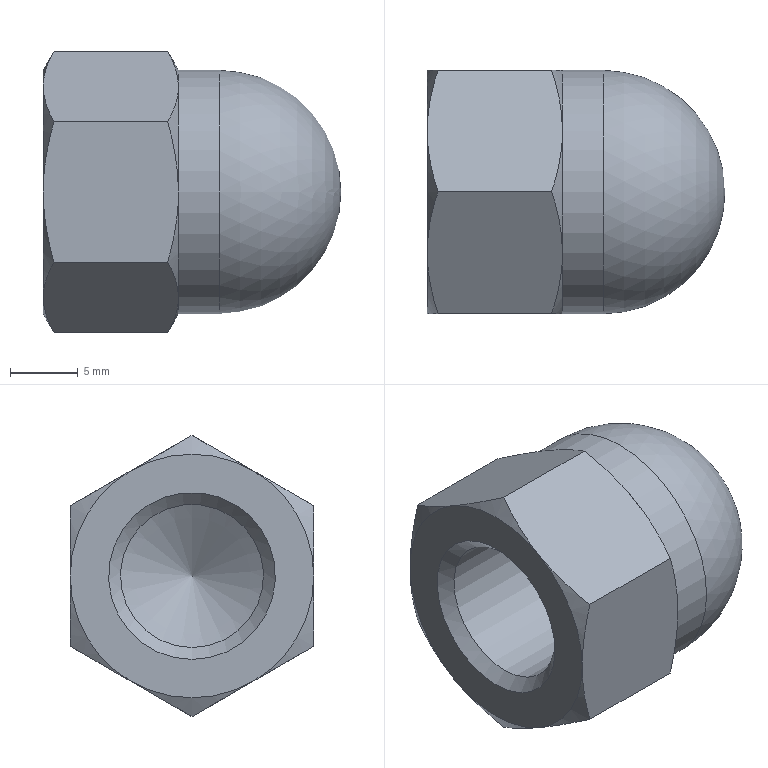Part | STEP file | Tube feed_id718_x_t | 1 solid | 27 faces | box 22 x 18 x 20.785 mm | volume 3414 mm3 | cone 15 | plane 8 | cylinder 3 | sphere 1 | commonest cylinder face diameters 10.579 x1 13 x1 18 x1